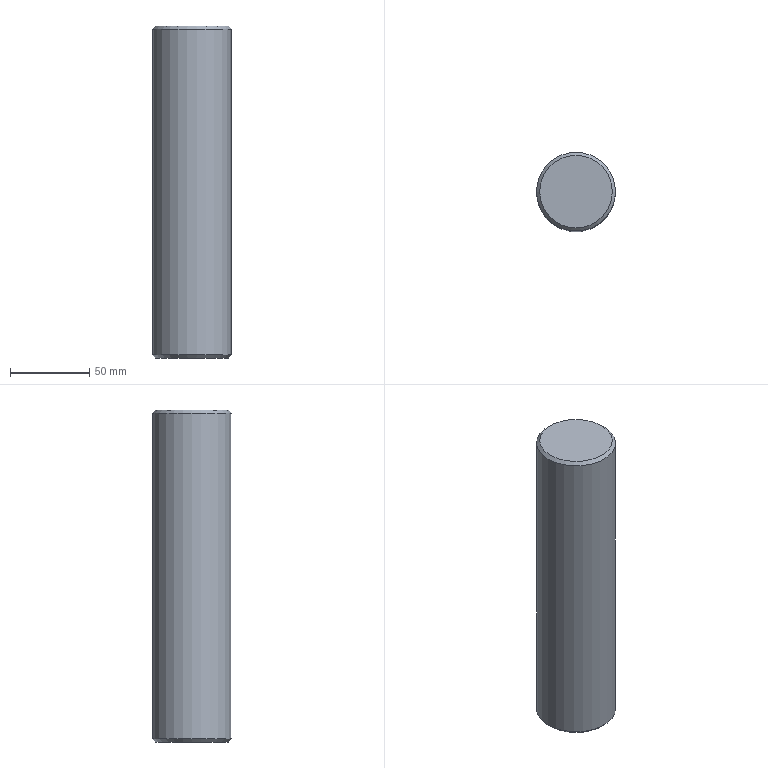Part | STEP file | 车灯-后视镜_id286_x_t | 1 solid | 9 faces | box 50 x 50 x 210 mm | volume 409927 mm3 | plane 3 | cylinder 3 | cone 3 | commonest cylinder face diameters 8.6 x1 10 x1 50 x1
STEP:
#1=CARTESIAN_POINT('',(87.,75.,-160.5));
#2=VERTEX_POINT('',#1);
#3=CARTESIAN_POINT('',(110.,75.,-160.5));
#4=DIRECTION('',(0.,0.,-1.));
#5=DIRECTION('',(-1.,0.,0.));
#6=AXIS2_PLACEMENT_3D('',#3,#4,#5);
#7=CIRCLE('',#6,23.);
#8=EDGE_CURVE('',#2,#2,#7,.T.);
#9=ORIENTED_EDGE('',*,*,#8,.F.);
#10=EDGE_LOOP('',(#9));
#11=FACE_OUTER_BOUND('',#10,.T.);
#12=CARTESIAN_POINT('',(110.,75.,-160.5));
#13=DIRECTION('',(0.,0.,1.));
#14=DIRECTION('',(-1.,0.,0.));
#15=AXIS2_PLACEMENT_3D('',#12,#13,#14);
#16=PLANE('',#15);
#17=ADVANCED_FACE('',(#11),#16,.T.);
#18=CARTESIAN_POINT('',(133.,75.,-370.5));
#19=VERTEX_POINT('',#18);
#20=CARTESIAN_POINT('',(110.,75.,-370.5));
#21=DIRECTION('',(0.,0.,1.));
#22=DIRECTION('',(1.,0.,0.));
#23=AXIS2_PLACEMENT_3D('',#20,#21,#22);
#24=CIRCLE('',#23,23.);
#25=EDGE_CURVE('',#19,#19,#24,.T.);
#26=ORIENTED_EDGE('',*,*,#25,.F.);
#27=EDGE_LOOP('',(#26));
#28=FACE_BOUND('',#27,.T.);
#29=CARTESIAN_POINT('',(105.,75.,-370.5));
#30=VERTEX_POINT('',#29);
#31=CARTESIAN_POINT('',(110.,75.,-370.5));
#32=DIRECTION('',(0.,0.,-1.));
#33=DIRECTION('',(-1.,0.,0.));
#34=AXIS2_PLACEMENT_3D('',#31,#32,#33);
#35=CIRCLE('',#34,5.);
#36=EDGE_CURVE('',#30,#30,#35,.T.);
#37=ORIENTED_EDGE('',*,*,#36,.F.);
#38=EDGE_LOOP('',(#37));
#39=FACE_BOUND('',#38,.T.);
#40=CARTESIAN_POINT('',(110.,75.,-370.5));
#41=DIRECTION('',(0.,0.,-1.));
#42=DIRECTION('',(1.,0.,0.));
#43=AXIS2_PLACEMENT_3D('',#40,#41,#42);
#44=PLANE('',#43);
#45=ADVANCED_FACE('',(#28,#39),#44,.T.);
#46=CARTESIAN_POINT('',(85.,75.,-162.5));
#47=VERTEX_POINT('',#46);
#48=CARTESIAN_POINT('',(110.,75.,-162.5));
#49=DIRECTION('',(0.,0.,1.));
#50=DIRECTION('',(-1.,0.,0.));
#51=AXIS2_PLACEMENT_3D('',#48,#49,#50);
#52=CIRCLE('',#51,25.);
#53=EDGE_CURVE('',#47,#47,#52,.T.);
#54=ORIENTED_EDGE('',*,*,#53,.F.);
#55=EDGE_LOOP('',(#54));
#56=FACE_BOUND('',#55,.T.);
#57=CARTESIAN_POINT('',(135.,75.,-368.5));
#58=VERTEX_POINT('',#57);
#59=CARTESIAN_POINT('',(110.,75.,-368.5));
#60=DIRECTION('',(0.,0.,-1.));
#61=DIRECTION('',(1.,0.,0.));
#62=AXIS2_PLACEMENT_3D('',#59,#60,#61);
#63=CIRCLE('',#62,25.);
#64=EDGE_CURVE('',#58,#58,#63,.T.);
#65=ORIENTED_EDGE('',*,*,#64,.F.);
#66=EDGE_LOOP('',(#65));
#67=FACE_BOUND('',#66,.T.);
#68=CARTESIAN_POINT('',(110.,75.,-330.5));
#69=DIRECTION('',(0.,0.,1.));
#70=DIRECTION('',(-1.,0.,0.));
#71=AXIS2_PLACEMENT_3D('',#68,#69,#70);
#72=CYLINDRICAL_SURFACE('',#71,25.);
#73=ADVANCED_FACE('',(#56,#67),#72,.T.);
#74=CARTESIAN_POINT('',(114.3,75.,-347.5));
#75=VERTEX_POINT('',#74);
#76=CARTESIAN_POINT('',(110.,75.,-347.5));
#77=DIRECTION('',(0.,0.,1.));
#78=DIRECTION('',(1.,0.,0.));
#79=AXIS2_PLACEMENT_3D('',#76,#77,#78);
#80=CIRCLE('',#79,4.3);
#81=EDGE_CURVE('',#75,#75,#80,.T.);
#82=ORIENTED_EDGE('',*,*,#81,.T.);
#83=EDGE_LOOP('',(#82));
#84=FACE_BOUND('',#83,.T.);
#85=CARTESIAN_POINT('',(105.7,75.,-350.5));
#86=VERTEX_POINT('',#85);
#87=CARTESIAN_POINT('',(110.,75.,-350.5));
#88=DIRECTION('',(0.,0.,1.));
#89=DIRECTION('',(-1.,0.,0.));
#90=AXIS2_PLACEMENT_3D('',#87,#88,#89);
#91=CIRCLE('',#90,4.3);
#92=EDGE_CURVE('',#86,#86,#91,.T.);
#93=ORIENTED_EDGE('',*,*,#92,.F.);
#94=EDGE_LOOP('',(#93));
#95=FACE_BOUND('',#94,.T.);
#96=CARTESIAN_POINT('',(110.,75.,-350.5));
#97=DIRECTION('',(0.,0.,1.));
#98=DIRECTION('',(-1.,0.,0.));
#99=AXIS2_PLACEMENT_3D('',#96,#97,#98);
#100=CYLINDRICAL_SURFACE('',#99,4.3);
#101=ADVANCED_FACE('',(#84,#95),#100,.F.);
#102=ORIENTED_EDGE('',*,*,#81,.F.);
#103=EDGE_LOOP('',(#102));
#104=FACE_BOUND('',#103,.T.);
#105=CARTESIAN_POINT('',(110.,75.,-344.916));
#106=VERTEX_POINT('',#105);
#107=VERTEX_LOOP('',#106);
#108=FACE_BOUND('',#107,.T.);
#109=CARTESIAN_POINT('',(110.,75.,-344.916));
#110=DIRECTION('',(0.,0.,-1.));
#111=DIRECTION('',(1.,0.,0.));
#112=AXIS2_PLACEMENT_3D('',#109,#110,#111);
#113=CONICAL_SURFACE('',#112,0.,59.);
#114=ADVANCED_FACE('',(#104,#108),#113,.F.);
#115=ORIENTED_EDGE('',*,*,#92,.T.);
#116=EDGE_LOOP('',(#115));
#117=FACE_BOUND('',#116,.T.);
#118=CARTESIAN_POINT('',(115.,75.,-350.5));
#119=VERTEX_POINT('',#118);
#120=CARTESIAN_POINT('',(110.,75.,-350.5));
#121=DIRECTION('',(0.,0.,1.));
#122=DIRECTION('',(1.,0.,0.));
#123=AXIS2_PLACEMENT_3D('',#120,#121,#122);
#124=CIRCLE('',#123,5.);
#125=EDGE_CURVE('',#119,#119,#124,.T.);
#126=ORIENTED_EDGE('',*,*,#125,.F.);
#127=EDGE_LOOP('',(#126));
#128=FACE_BOUND('',#127,.T.);
#129=CARTESIAN_POINT('',(110.,75.,-350.5));
#130=DIRECTION('',(0.,0.,1.));
#131=DIRECTION('',(-1.,0.,0.));
#132=AXIS2_PLACEMENT_3D('',#129,#130,#131);
#133=PLANE('',#132);
#134=ADVANCED_FACE('',(#117,#128),#133,.F.);
#135=ORIENTED_EDGE('',*,*,#125,.T.);
#136=EDGE_LOOP('',(#135));
#137=FACE_BOUND('',#136,.T.);
#138=ORIENTED_EDGE('',*,*,#36,.T.);
#139=EDGE_LOOP('',(#138));
#140=FACE_BOUND('',#139,.T.);
#141=CARTESIAN_POINT('',(110.,75.,-370.5));
#142=DIRECTION('',(0.,0.,1.));
#143=DIRECTION('',(-1.,0.,0.));
#144=AXIS2_PLACEMENT_3D('',#141,#142,#143);
#145=CYLINDRICAL_SURFACE('',#144,5.);
#146=ADVANCED_FACE('',(#137,#140),#145,.F.);
#147=ORIENTED_EDGE('',*,*,#25,.T.);
#148=EDGE_LOOP('',(#147));
#149=FACE_BOUND('',#148,.T.);
#150=ORIENTED_EDGE('',*,*,#64,.T.);
#151=EDGE_LOOP('',(#150));
#152=FACE_BOUND('',#151,.T.);
#153=CARTESIAN_POINT('',(110.,75.,-368.5));
#154=DIRECTION('',(0.,0.,1.));
#155=DIRECTION('',(-1.,0.,0.));
#156=AXIS2_PLACEMENT_3D('',#153,#154,#155);
#157=CONICAL_SURFACE('',#156,25.,45.);
#158=ADVANCED_FACE('',(#149,#152),#157,.T.);
#159=ORIENTED_EDGE('',*,*,#8,.T.);
#160=EDGE_LOOP('',(#159));
#161=FACE_BOUND('',#160,.T.);
#162=ORIENTED_EDGE('',*,*,#53,.T.);
#163=EDGE_LOOP('',(#162));
#164=FACE_BOUND('',#163,.T.);
#165=CARTESIAN_POINT('',(110.,75.,-162.5));
#166=DIRECTION('',(0.,0.,-1.));
#167=DIRECTION('',(1.,0.,0.));
#168=AXIS2_PLACEMENT_3D('',#165,#166,#167);
#169=CONICAL_SURFACE('',#168,25.,45.);
#170=ADVANCED_FACE('',(#161,#164),#169,.T.);
#171=CLOSED_SHELL('',(#17,#45,#73,#101,#114,#134,#146,#158,#170));
#172=MANIFOLD_SOLID_BREP('',#171);
#173=(LENGTH_UNIT()NAMED_UNIT(*)SI_UNIT(.MILLI.,.METRE.));
#174=UNCERTAINTY_MEASURE_WITH_UNIT(LENGTH_MEASURE(0.00002),#173,'','');
#175=(NAMED_UNIT(*)PLANE_ANGLE_UNIT()SI_UNIT($,.RADIAN.));
#176=PLANE_ANGLE_MEASURE_WITH_UNIT(PLANE_ANGLE_MEASURE(0.01745),#175);
#177=DIMENSIONAL_EXPONENTS(0.,0.,0.,0.,0.,0.,0.);
#178=(CONVERSION_BASED_UNIT('DEGREE',#176)NAMED_UNIT(#177)PLANE_ANGLE_UNIT());
#179=(NAMED_UNIT(*)SI_UNIT($,.STERADIAN.)SOLID_ANGLE_UNIT());
#180=(GEOMETRIC_REPRESENTATION_CONTEXT(3)GLOBAL_UNCERTAINTY_ASSIGNED_CONTEXT((#174))GLOBAL_UNIT_ASSIGNED_CONTEXT((#173,#178,#179))REPRESENTATION_CONTEXT('',''));
#181=ADVANCED_BREP_SHAPE_REPRESENTATION('',(#172),#180);